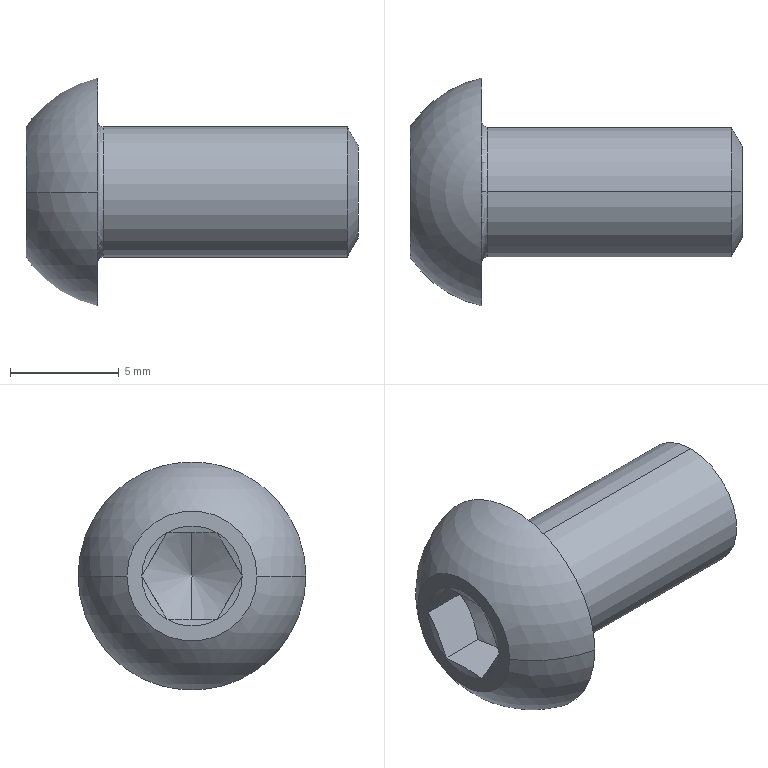Part | SolidWorks | features RevCut 2, Revolution 2, Cut 1, LPattern 1, RefAxis 1 | 1 solid | 25 faces | box 15.3 x 10.5 x 10.5 mm | volume 508.665 mm3 | cone 10 | plane 9 | torus 2 | sphere 2 | cylinder 2 | commonest cylinder face diameters 6 x2
STEP:
#1=CARTESIAN_POINT('',(0.,0.,2.134));
#2=VERTEX_POINT('',#1);
#3=CARTESIAN_POINT('',(0.,0.,-2.134));
#4=VERTEX_POINT('',#3);
#5=CARTESIAN_POINT('',(0.,0.,0.));
#6=DIRECTION('',(-1.,0.,0.));
#7=DIRECTION('',(0.,0.,1.));
#8=AXIS2_PLACEMENT_3D('',#5,#6,#7);
#9=CIRCLE('',#8,2.134);
#10=EDGE_CURVE('',#2,#4,#9,.T.);
#11=ORIENTED_EDGE('',*,*,#10,.T.);
#12=CARTESIAN_POINT('',(-0.5,0.,-3.));
#13=VERTEX_POINT('',#12);
#14=CARTESIAN_POINT('',(-0.5,0.,-3.));
#15=DIRECTION('',(-0.5,0.,-0.866));
#16=VECTOR('',#15,1000.);
#17=LINE('',#14,#16);
#18=EDGE_CURVE('',#4,#13,#17,.T.);
#19=ORIENTED_EDGE('',*,*,#18,.T.);
#20=CARTESIAN_POINT('',(-0.5,0.,3.));
#21=VERTEX_POINT('',#20);
#22=CARTESIAN_POINT('',(-0.5,0.,0.));
#23=DIRECTION('',(-1.,0.,0.));
#24=DIRECTION('',(0.,0.,1.));
#25=AXIS2_PLACEMENT_3D('',#22,#23,#24);
#26=CIRCLE('',#25,3.);
#27=EDGE_CURVE('',#21,#13,#26,.T.);
#28=ORIENTED_EDGE('',*,*,#27,.F.);
#29=CARTESIAN_POINT('',(-0.5,0.,3.));
#30=DIRECTION('',(-0.5,0.,0.866));
#31=VECTOR('',#30,1000.);
#32=LINE('',#29,#31);
#33=EDGE_CURVE('',#2,#21,#32,.T.);
#34=ORIENTED_EDGE('',*,*,#33,.F.);
#35=EDGE_LOOP('',(#11,#19,#28,#34));
#36=FACE_OUTER_BOUND('',#35,.T.);
#37=CARTESIAN_POINT('',(-0.5,0.,0.));
#38=DIRECTION('',(-1.,0.,0.));
#39=DIRECTION('',(0.,0.,1.));
#40=AXIS2_PLACEMENT_3D('',#37,#38,#39);
#41=CONICAL_SURFACE('',#40,3.,1.047);
#42=ADVANCED_FACE('',(#36),#41,.T.);
#43=CARTESIAN_POINT('',(-12.,0.,0.));
#44=VERTEX_POINT('',#43);
#45=CARTESIAN_POINT('',(-13.057,0.,2.));
#46=VERTEX_POINT('',#45);
#47=CARTESIAN_POINT('',(-13.22,0.,2.309));
#48=DIRECTION('',(-0.4671,0.,0.8842));
#49=VECTOR('',#48,1000.);
#50=LINE('',#47,#49);
#51=EDGE_CURVE('',#44,#46,#50,.T.);
#52=ORIENTED_EDGE('',*,*,#51,.F.);
#53=CARTESIAN_POINT('',(-13.057,0.,-2.));
#54=VERTEX_POINT('',#53);
#55=CARTESIAN_POINT('',(-13.22,0.,-2.309));
#56=DIRECTION('',(-0.4671,0.,-0.8842));
#57=VECTOR('',#56,1000.);
#58=LINE('',#55,#57);
#59=EDGE_CURVE('',#44,#54,#58,.T.);
#60=ORIENTED_EDGE('',*,*,#59,.T.);
#61=CARTESIAN_POINT('',(-13.22,-1.155,-2.));
#62=VERTEX_POINT('',#61);
#63=CARTESIAN_POINT('',(-13.057,0.,-2.));
#64=CARTESIAN_POINT('',(-13.057,-0.1946,-2.));
#65=CARTESIAN_POINT('',(-13.072,-0.3883,-2.));
#66=CARTESIAN_POINT('',(-13.129,-0.774,-2.));
#67=CARTESIAN_POINT('',(-13.17,-0.9664,-2.));
#68=CARTESIAN_POINT('',(-13.22,-1.155,-2.));
#69=B_SPLINE_CURVE_WITH_KNOTS('',3,(#63,#64,#65,#66,#67,#68),.UNSPECIFIED.,.F.,.F.,(4,2,4),(0.002255,0.002836,0.003416),.UNSPECIFIED.);
#70=EDGE_CURVE('',#54,#62,#69,.T.);
#71=ORIENTED_EDGE('',*,*,#70,.T.);
#72=CARTESIAN_POINT('',(-13.22,-2.309,0.));
#73=VERTEX_POINT('',#72);
#74=CARTESIAN_POINT('',(-13.22,-1.155,-2.));
#75=CARTESIAN_POINT('',(-13.12,-1.344,-1.672));
#76=CARTESIAN_POINT('',(-13.057,-1.535,-1.341));
#77=CARTESIAN_POINT('',(-13.056,-1.927,-0.6622));
#78=CARTESIAN_POINT('',(-13.12,-2.12,-0.3279));
#79=CARTESIAN_POINT('',(-13.22,-2.309,0.));
#80=B_SPLINE_CURVE_WITH_KNOTS('',3,(#74,#75,#76,#77,#78,#79),.UNSPECIFIED.,.F.,.F.,(4,2,4),(0.000000237,0.001165,0.002329),.UNSPECIFIED.);
#81=EDGE_CURVE('',#62,#73,#80,.T.);
#82=ORIENTED_EDGE('',*,*,#81,.T.);
#83=CARTESIAN_POINT('',(-13.22,-1.155,2.));
#84=VERTEX_POINT('',#83);
#85=CARTESIAN_POINT('',(-13.22,-2.309,0.));
#86=CARTESIAN_POINT('',(-13.12,-2.12,0.3276));
#87=CARTESIAN_POINT('',(-13.057,-1.929,0.6595));
#88=CARTESIAN_POINT('',(-13.056,-1.537,1.338));
#89=CARTESIAN_POINT('',(-13.12,-1.344,1.672));
#90=CARTESIAN_POINT('',(-13.22,-1.155,2.));
#91=B_SPLINE_CURVE_WITH_KNOTS('',3,(#85,#86,#87,#88,#89,#90),.UNSPECIFIED.,.F.,.F.,(4,2,4),(0.000000237,0.001165,0.002329),.UNSPECIFIED.);
#92=EDGE_CURVE('',#73,#84,#91,.T.);
#93=ORIENTED_EDGE('',*,*,#92,.T.);
#94=CARTESIAN_POINT('',(-13.22,-1.155,2.));
#95=CARTESIAN_POINT('',(-13.17,-0.9664,2.));
#96=CARTESIAN_POINT('',(-13.129,-0.774,2.));
#97=CARTESIAN_POINT('',(-13.072,-0.3883,2.));
#98=CARTESIAN_POINT('',(-13.057,-0.1946,2.));
#99=CARTESIAN_POINT('',(-13.057,0.,2.));
#100=B_SPLINE_CURVE_WITH_KNOTS('',3,(#94,#95,#96,#97,#98,#99),.UNSPECIFIED.,.F.,.F.,(4,2,4),(0.001973,0.002555,0.003138),.UNSPECIFIED.);
#101=EDGE_CURVE('',#84,#46,#100,.T.);
#102=ORIENTED_EDGE('',*,*,#101,.T.);
#103=EDGE_LOOP('',(#52,#60,#71,#82,#93,#102));
#104=FACE_OUTER_BOUND('',#103,.T.);
#105=CARTESIAN_POINT('',(-13.22,0.,0.));
#106=DIRECTION('',(-1.,0.,0.));
#107=DIRECTION('',(0.,0.,1.));
#108=AXIS2_PLACEMENT_3D('',#105,#106,#107);
#109=CONICAL_SURFACE('',#108,2.309,1.085);
#110=ADVANCED_FACE('',(#104),#109,.F.);
#111=CARTESIAN_POINT('',(-12.,0.,-3.25));
#112=VERTEX_POINT('',#111);
#113=CARTESIAN_POINT('',(-12.,0.,3.25));
#114=VERTEX_POINT('',#113);
#115=CARTESIAN_POINT('',(-12.,0.,0.));
#116=DIRECTION('',(-1.,0.,0.));
#117=DIRECTION('',(0.,0.,1.));
#118=AXIS2_PLACEMENT_3D('',#115,#116,#117);
#119=CIRCLE('',#118,3.25);
#120=EDGE_CURVE('',#112,#114,#119,.T.);
#121=ORIENTED_EDGE('',*,*,#120,.F.);
#122=CARTESIAN_POINT('',(-11.75,0.,-3.));
#123=VERTEX_POINT('',#122);
#124=CARTESIAN_POINT('',(-11.75,0.,-3.25));
#125=DIRECTION('',(0.,1.,0.));
#126=DIRECTION('',(0.,0.,1.));
#127=AXIS2_PLACEMENT_3D('',#124,#125,#126);
#128=CIRCLE('',#127,0.25);
#129=EDGE_CURVE('',#112,#123,#128,.T.);
#130=ORIENTED_EDGE('',*,*,#129,.T.);
#131=CARTESIAN_POINT('',(-11.75,0.,3.));
#132=VERTEX_POINT('',#131);
#133=CARTESIAN_POINT('',(-11.75,0.,0.));
#134=DIRECTION('',(-1.,0.,0.));
#135=DIRECTION('',(0.,0.,1.));
#136=AXIS2_PLACEMENT_3D('',#133,#134,#135);
#137=CIRCLE('',#136,3.);
#138=EDGE_CURVE('',#123,#132,#137,.T.);
#139=ORIENTED_EDGE('',*,*,#138,.T.);
#140=CARTESIAN_POINT('',(-11.75,0.,3.25));
#141=DIRECTION('',(0.,-1.,0.));
#142=DIRECTION('',(0.,0.,-1.));
#143=AXIS2_PLACEMENT_3D('',#140,#141,#142);
#144=CIRCLE('',#143,0.25);
#145=EDGE_CURVE('',#114,#132,#144,.T.);
#146=ORIENTED_EDGE('',*,*,#145,.F.);
#147=EDGE_LOOP('',(#121,#130,#139,#146));
#148=FACE_OUTER_BOUND('',#147,.T.);
#149=CARTESIAN_POINT('',(-11.75,0.,0.));
#150=DIRECTION('',(-1.,0.,0.));
#151=DIRECTION('',(0.,0.,1.));
#152=AXIS2_PLACEMENT_3D('',#149,#150,#151);
#153=TOROIDAL_SURFACE('',#152,3.25,0.25);
#154=ADVANCED_FACE('',(#148),#153,.F.);
#155=CARTESIAN_POINT('',(-12.,5.25,0.));
#156=VERTEX_POINT('',#155);
#157=CARTESIAN_POINT('',(-12.,-5.25,0.));
#158=VERTEX_POINT('',#157);
#159=CARTESIAN_POINT('',(-12.,0.,0.));
#160=DIRECTION('',(-1.,0.,0.));
#161=DIRECTION('',(0.,0.,1.));
#162=AXIS2_PLACEMENT_3D('',#159,#160,#161);
#163=CIRCLE('',#162,5.25);
#164=EDGE_CURVE('',#156,#158,#163,.T.);
#165=ORIENTED_EDGE('',*,*,#164,.T.);
#166=CARTESIAN_POINT('',(-15.3,-3.,0.));
#167=VERTEX_POINT('',#166);
#168=CARTESIAN_POINT('',(-10.838,0.,0.));
#169=DIRECTION('',(0.,0.,-1.));
#170=DIRECTION('',(0.,1.,0.));
#171=AXIS2_PLACEMENT_3D('',#168,#169,#170);
#172=CIRCLE('',#171,5.377);
#173=EDGE_CURVE('',#158,#167,#172,.T.);
#174=ORIENTED_EDGE('',*,*,#173,.T.);
#175=CARTESIAN_POINT('',(-15.3,3.,0.));
#176=VERTEX_POINT('',#175);
#177=CARTESIAN_POINT('',(-15.3,0.,0.));
#178=DIRECTION('',(-1.,0.,0.));
#179=DIRECTION('',(0.,0.,1.));
#180=AXIS2_PLACEMENT_3D('',#177,#178,#179);
#181=CIRCLE('',#180,3.);
#182=EDGE_CURVE('',#176,#167,#181,.T.);
#183=ORIENTED_EDGE('',*,*,#182,.F.);
#184=CARTESIAN_POINT('',(-10.838,0.,0.));
#185=DIRECTION('',(0.,0.,1.));
#186=DIRECTION('',(1.,0.,0.));
#187=AXIS2_PLACEMENT_3D('',#184,#185,#186);
#188=CIRCLE('',#187,5.377);
#189=EDGE_CURVE('',#156,#176,#188,.T.);
#190=ORIENTED_EDGE('',*,*,#189,.F.);
#191=EDGE_LOOP('',(#165,#174,#183,#190));
#192=FACE_OUTER_BOUND('',#191,.T.);
#193=CARTESIAN_POINT('',(-10.838,0.,0.));
#194=DIRECTION('',(0.,0.,-1.));
#195=DIRECTION('',(0.,1.,0.));
#196=AXIS2_PLACEMENT_3D('',#193,#194,#195);
#197=SPHERICAL_SURFACE('',#196,5.377);
#198=ADVANCED_FACE('',(#192),#197,.T.);
#199=ORIENTED_EDGE('',*,*,#27,.T.);
#200=CARTESIAN_POINT('',(-15.3,0.,-3.));
#201=DIRECTION('',(-1.,0.,0.));
#202=VECTOR('',#201,1000.);
#203=LINE('',#200,#202);
#204=EDGE_CURVE('',#13,#123,#203,.T.);
#205=ORIENTED_EDGE('',*,*,#204,.T.);
#206=CARTESIAN_POINT('',(-11.75,0.,0.));
#207=DIRECTION('',(-1.,0.,0.));
#208=DIRECTION('',(0.,0.,1.));
#209=AXIS2_PLACEMENT_3D('',#206,#207,#208);
#210=CIRCLE('',#209,3.);
#211=EDGE_CURVE('',#132,#123,#210,.T.);
#212=ORIENTED_EDGE('',*,*,#211,.F.);
#213=CARTESIAN_POINT('',(-15.3,0.,3.));
#214=DIRECTION('',(-1.,0.,0.));
#215=VECTOR('',#214,1000.);
#216=LINE('',#213,#215);
#217=EDGE_CURVE('',#21,#132,#216,.T.);
#218=ORIENTED_EDGE('',*,*,#217,.F.);
#219=EDGE_LOOP('',(#199,#205,#212,#218));
#220=FACE_OUTER_BOUND('',#219,.T.);
#221=CARTESIAN_POINT('',(-15.3,0.,0.));
#222=DIRECTION('',(-1.,0.,0.));
#223=DIRECTION('',(0.,0.,1.));
#224=AXIS2_PLACEMENT_3D('',#221,#222,#223);
#225=CYLINDRICAL_SURFACE('',#224,3.);
#226=ADVANCED_FACE('',(#220),#225,.T.);
#227=ORIENTED_EDGE('',*,*,#204,.F.);
#228=CARTESIAN_POINT('',(-0.5,0.,0.));
#229=DIRECTION('',(-1.,0.,0.));
#230=DIRECTION('',(0.,0.,1.));
#231=AXIS2_PLACEMENT_3D('',#228,#229,#230);
#232=CIRCLE('',#231,3.);
#233=EDGE_CURVE('',#13,#21,#232,.T.);
#234=ORIENTED_EDGE('',*,*,#233,.T.);
#235=ORIENTED_EDGE('',*,*,#217,.T.);
#236=ORIENTED_EDGE('',*,*,#138,.F.);
#237=EDGE_LOOP('',(#227,#234,#235,#236));
#238=FACE_OUTER_BOUND('',#237,.T.);
#239=CARTESIAN_POINT('',(-15.3,0.,0.));
#240=DIRECTION('',(-1.,0.,0.));
#241=DIRECTION('',(0.,0.,1.));
#242=AXIS2_PLACEMENT_3D('',#239,#240,#241);
#243=CYLINDRICAL_SURFACE('',#242,3.);
#244=ADVANCED_FACE('',(#238),#243,.T.);
#245=ORIENTED_EDGE('',*,*,#182,.T.);
#246=CARTESIAN_POINT('',(-15.3,0.,0.));
#247=DIRECTION('',(-1.,0.,0.));
#248=DIRECTION('',(0.,0.,1.));
#249=AXIS2_PLACEMENT_3D('',#246,#247,#248);
#250=CIRCLE('',#249,3.);
#251=EDGE_CURVE('',#167,#176,#250,.T.);
#252=ORIENTED_EDGE('',*,*,#251,.T.);
#253=EDGE_LOOP('',(#245,#252));
#254=FACE_OUTER_BOUND('',#253,.T.);
#255=CARTESIAN_POINT('',(-15.3,-1.155,-2.));
#256=VERTEX_POINT('',#255);
#257=CARTESIAN_POINT('',(-15.3,-2.309,0.));
#258=VERTEX_POINT('',#257);
#259=CARTESIAN_POINT('',(-15.3,0.,0.));
#260=DIRECTION('',(-1.,0.,0.));
#261=DIRECTION('',(0.,0.,-1.));
#262=AXIS2_PLACEMENT_3D('',#259,#260,#261);
#263=CIRCLE('',#262,2.309);
#264=EDGE_CURVE('',#256,#258,#263,.T.);
#265=ORIENTED_EDGE('',*,*,#264,.F.);
#266=CARTESIAN_POINT('',(-15.3,1.155,-2.));
#267=VERTEX_POINT('',#266);
#268=CARTESIAN_POINT('',(-15.3,0.,0.));
#269=DIRECTION('',(-1.,0.,0.));
#270=DIRECTION('',(0.,0.,-1.));
#271=AXIS2_PLACEMENT_3D('',#268,#269,#270);
#272=CIRCLE('',#271,2.309);
#273=EDGE_CURVE('',#267,#256,#272,.T.);
#274=ORIENTED_EDGE('',*,*,#273,.F.);
#275=CARTESIAN_POINT('',(-15.3,2.309,0.));
#276=VERTEX_POINT('',#275);
#277=CARTESIAN_POINT('',(-15.3,0.,0.));
#278=DIRECTION('',(-1.,0.,0.));
#279=DIRECTION('',(0.,0.,-1.));
#280=AXIS2_PLACEMENT_3D('',#277,#278,#279);
#281=CIRCLE('',#280,2.309);
#282=EDGE_CURVE('',#276,#267,#281,.T.);
#283=ORIENTED_EDGE('',*,*,#282,.F.);
#284=CARTESIAN_POINT('',(-15.3,1.155,2.));
#285=VERTEX_POINT('',#284);
#286=CARTESIAN_POINT('',(-15.3,0.,0.));
#287=DIRECTION('',(-1.,0.,0.));
#288=DIRECTION('',(0.,0.,-1.));
#289=AXIS2_PLACEMENT_3D('',#286,#287,#288);
#290=CIRCLE('',#289,2.309);
#291=EDGE_CURVE('',#285,#276,#290,.T.);
#292=ORIENTED_EDGE('',*,*,#291,.F.);
#293=CARTESIAN_POINT('',(-15.3,-1.155,2.));
#294=VERTEX_POINT('',#293);
#295=CARTESIAN_POINT('',(-15.3,0.,0.));
#296=DIRECTION('',(-1.,0.,0.));
#297=DIRECTION('',(0.,0.,-1.));
#298=AXIS2_PLACEMENT_3D('',#295,#296,#297);
#299=CIRCLE('',#298,2.309);
#300=EDGE_CURVE('',#294,#285,#299,.T.);
#301=ORIENTED_EDGE('',*,*,#300,.F.);
#302=CARTESIAN_POINT('',(-15.3,0.,0.));
#303=DIRECTION('',(-1.,0.,0.));
#304=DIRECTION('',(0.,-1.,0.));
#305=AXIS2_PLACEMENT_3D('',#302,#303,#304);
#306=CIRCLE('',#305,2.309);
#307=EDGE_CURVE('',#258,#294,#306,.T.);
#308=ORIENTED_EDGE('',*,*,#307,.F.);
#309=EDGE_LOOP('',(#265,#274,#283,#292,#301,#308));
#310=FACE_BOUND('',#309,.T.);
#311=CARTESIAN_POINT('',(-15.3,0.,0.));
#312=DIRECTION('',(1.,0.,0.));
#313=DIRECTION('',(0.,0.,-1.));
#314=AXIS2_PLACEMENT_3D('',#311,#312,#313);
#315=PLANE('',#314);
#316=ADVANCED_FACE('',(#254,#310),#315,.F.);
#317=ORIENTED_EDGE('',*,*,#173,.F.);
#318=CARTESIAN_POINT('',(-12.,0.,0.));
#319=DIRECTION('',(-1.,0.,0.));
#320=DIRECTION('',(0.,0.,1.));
#321=AXIS2_PLACEMENT_3D('',#318,#319,#320);
#322=CIRCLE('',#321,5.25);
#323=EDGE_CURVE('',#158,#156,#322,.T.);
#324=ORIENTED_EDGE('',*,*,#323,.T.);
#325=ORIENTED_EDGE('',*,*,#189,.T.);
#326=ORIENTED_EDGE('',*,*,#251,.F.);
#327=EDGE_LOOP('',(#317,#324,#325,#326));
#328=FACE_OUTER_BOUND('',#327,.T.);
#329=CARTESIAN_POINT('',(-10.838,0.,0.));
#330=DIRECTION('',(0.,0.,-1.));
#331=DIRECTION('',(0.,1.,0.));
#332=AXIS2_PLACEMENT_3D('',#329,#330,#331);
#333=SPHERICAL_SURFACE('',#332,5.377);
#334=ADVANCED_FACE('',(#328),#333,.T.);
#335=ORIENTED_EDGE('',*,*,#164,.F.);
#336=ORIENTED_EDGE('',*,*,#323,.F.);
#337=EDGE_LOOP('',(#335,#336));
#338=FACE_OUTER_BOUND('',#337,.T.);
#339=CARTESIAN_POINT('',(-12.,0.,0.));
#340=DIRECTION('',(-1.,0.,0.));
#341=DIRECTION('',(0.,0.,1.));
#342=AXIS2_PLACEMENT_3D('',#339,#340,#341);
#343=CIRCLE('',#342,3.25);
#344=EDGE_CURVE('',#114,#112,#343,.T.);
#345=ORIENTED_EDGE('',*,*,#344,.T.);
#346=ORIENTED_EDGE('',*,*,#120,.T.);
#347=EDGE_LOOP('',(#345,#346));
#348=FACE_BOUND('',#347,.T.);
#349=CARTESIAN_POINT('',(-12.,3.25,0.));
#350=DIRECTION('',(-1.,0.,0.));
#351=DIRECTION('',(0.,0.,1.));
#352=AXIS2_PLACEMENT_3D('',#349,#350,#351);
#353=PLANE('',#352);
#354=ADVANCED_FACE('',(#338,#348),#353,.F.);
#355=ORIENTED_EDGE('',*,*,#129,.F.);
#356=ORIENTED_EDGE('',*,*,#344,.F.);
#357=ORIENTED_EDGE('',*,*,#145,.T.);
#358=ORIENTED_EDGE('',*,*,#211,.T.);
#359=EDGE_LOOP('',(#355,#356,#357,#358));
#360=FACE_OUTER_BOUND('',#359,.T.);
#361=CARTESIAN_POINT('',(-11.75,0.,0.));
#362=DIRECTION('',(-1.,0.,0.));
#363=DIRECTION('',(0.,0.,1.));
#364=AXIS2_PLACEMENT_3D('',#361,#362,#363);
#365=TOROIDAL_SURFACE('',#364,3.25,0.25);
#366=ADVANCED_FACE('',(#360),#365,.F.);
#367=CARTESIAN_POINT('',(-15.3,-1.155,-2.));
#368=CARTESIAN_POINT('',(-15.252,-0.7703,-2.));
#369=CARTESIAN_POINT('',(-15.222,-0.3832,-2.));
#370=CARTESIAN_POINT('',(-15.222,0.3869,-2.));
#371=CARTESIAN_POINT('',(-15.252,0.7711,-2.));
#372=CARTESIAN_POINT('',(-15.3,1.155,-2.));
#373=B_SPLINE_CURVE_WITH_KNOTS('',3,(#367,#368,#369,#370,#371,#372),.UNSPECIFIED.,.F.,.F.,(4,2,4),(0.001892,0.003053,0.004215),.UNSPECIFIED.);
#374=EDGE_CURVE('',#256,#267,#373,.T.);
#375=ORIENTED_EDGE('',*,*,#374,.T.);
#376=ORIENTED_EDGE('',*,*,#273,.T.);
#377=EDGE_LOOP('',(#375,#376));
#378=FACE_OUTER_BOUND('',#377,.T.);
#379=CARTESIAN_POINT('',(-1014.72,0.,0.));
#380=DIRECTION('',(-1.,0.,0.));
#381=DIRECTION('',(0.,-1.,0.));
#382=AXIS2_PLACEMENT_3D('',#379,#380,#381);
#383=CONICAL_SURFACE('',#382,3981.726,1.325);
#384=ADVANCED_FACE('',(#378),#383,.F.);
#385=CARTESIAN_POINT('',(-15.3,1.155,-2.));
#386=CARTESIAN_POINT('',(-15.252,1.347,-1.667));
#387=CARTESIAN_POINT('',(-15.193,1.732,-1.));
#388=CARTESIAN_POINT('',(-15.252,2.117,-0.3333));
#389=CARTESIAN_POINT('',(-15.3,2.309,0.));
#390=B_SPLINE_CURVE_WITH_KNOTS('',3,(#385,#386,#387,#388,#389),.UNSPECIFIED.,.F.,.F.,(4,1,4),(0.000000231,0.001155,0.00231),.UNSPECIFIED.);
#391=EDGE_CURVE('',#267,#276,#390,.T.);
#392=ORIENTED_EDGE('',*,*,#391,.T.);
#393=ORIENTED_EDGE('',*,*,#282,.T.);
#394=EDGE_LOOP('',(#392,#393));
#395=FACE_OUTER_BOUND('',#394,.T.);
#396=CARTESIAN_POINT('',(-1014.72,0.,0.));
#397=DIRECTION('',(-1.,0.,0.));
#398=DIRECTION('',(0.,-1.,0.));
#399=AXIS2_PLACEMENT_3D('',#396,#397,#398);
#400=CONICAL_SURFACE('',#399,3981.726,1.325);
#401=ADVANCED_FACE('',(#395),#400,.F.);
#402=CARTESIAN_POINT('',(-15.3,2.309,0.));
#403=CARTESIAN_POINT('',(-15.252,2.117,0.3333));
#404=CARTESIAN_POINT('',(-15.193,1.732,1.));
#405=CARTESIAN_POINT('',(-15.252,1.347,1.667));
#406=CARTESIAN_POINT('',(-15.3,1.155,2.));
#407=B_SPLINE_CURVE_WITH_KNOTS('',3,(#402,#403,#404,#405,#406),.UNSPECIFIED.,.F.,.F.,(4,1,4),(0.000000231,0.001155,0.00231),.UNSPECIFIED.);
#408=EDGE_CURVE('',#276,#285,#407,.T.);
#409=ORIENTED_EDGE('',*,*,#408,.T.);
#410=ORIENTED_EDGE('',*,*,#291,.T.);
#411=EDGE_LOOP('',(#409,#410));
#412=FACE_OUTER_BOUND('',#411,.T.);
#413=CARTESIAN_POINT('',(-1014.72,0.,0.));
#414=DIRECTION('',(-1.,0.,0.));
#415=DIRECTION('',(0.,-1.,0.));
#416=AXIS2_PLACEMENT_3D('',#413,#414,#415);
#417=CONICAL_SURFACE('',#416,3981.726,1.325);
#418=ADVANCED_FACE('',(#412),#417,.F.);
#419=CARTESIAN_POINT('',(-15.3,1.155,2.));
#420=CARTESIAN_POINT('',(-15.252,0.7711,2.));
#421=CARTESIAN_POINT('',(-15.222,0.3869,2.));
#422=CARTESIAN_POINT('',(-15.222,-0.3832,2.));
#423=CARTESIAN_POINT('',(-15.252,-0.7703,2.));
#424=CARTESIAN_POINT('',(-15.3,-1.155,2.));
#425=B_SPLINE_CURVE_WITH_KNOTS('',3,(#419,#420,#421,#422,#423,#424),.UNSPECIFIED.,.F.,.F.,(4,2,4),(0.004742,0.005901,0.007061),.UNSPECIFIED.);
#426=EDGE_CURVE('',#285,#294,#425,.T.);
#427=ORIENTED_EDGE('',*,*,#426,.T.);
#428=ORIENTED_EDGE('',*,*,#300,.T.);
#429=EDGE_LOOP('',(#427,#428));
#430=FACE_OUTER_BOUND('',#429,.T.);
#431=CARTESIAN_POINT('',(-1014.72,0.,0.));
#432=DIRECTION('',(-1.,0.,0.));
#433=DIRECTION('',(0.,-1.,0.));
#434=AXIS2_PLACEMENT_3D('',#431,#432,#433);
#435=CONICAL_SURFACE('',#434,3981.726,1.325);
#436=ADVANCED_FACE('',(#430),#435,.F.);
#437=CARTESIAN_POINT('',(-15.3,-1.155,2.));
#438=CARTESIAN_POINT('',(-15.252,-1.347,1.667));
#439=CARTESIAN_POINT('',(-15.193,-1.732,1.));
#440=CARTESIAN_POINT('',(-15.252,-2.117,0.3333));
#441=CARTESIAN_POINT('',(-15.3,-2.309,0.));
#442=B_SPLINE_CURVE_WITH_KNOTS('',3,(#437,#438,#439,#440,#441),.UNSPECIFIED.,.F.,.F.,(4,1,4),(0.000000231,0.001155,0.00231),.UNSPECIFIED.);
#443=EDGE_CURVE('',#294,#258,#442,.T.);
#444=ORIENTED_EDGE('',*,*,#443,.T.);
#445=ORIENTED_EDGE('',*,*,#307,.T.);
#446=EDGE_LOOP('',(#444,#445));
#447=FACE_OUTER_BOUND('',#446,.T.);
#448=CARTESIAN_POINT('',(-1014.72,0.,0.));
#449=DIRECTION('',(-1.,0.,0.));
#450=DIRECTION('',(0.,-1.,0.));
#451=AXIS2_PLACEMENT_3D('',#448,#449,#450);
#452=CONICAL_SURFACE('',#451,3981.726,1.325);
#453=ADVANCED_FACE('',(#447),#452,.F.);
#454=CARTESIAN_POINT('',(-15.3,-2.309,0.));
#455=CARTESIAN_POINT('',(-15.252,-2.117,-0.3333));
#456=CARTESIAN_POINT('',(-15.193,-1.732,-1.));
#457=CARTESIAN_POINT('',(-15.252,-1.347,-1.667));
#458=CARTESIAN_POINT('',(-15.3,-1.155,-2.));
#459=B_SPLINE_CURVE_WITH_KNOTS('',3,(#454,#455,#456,#457,#458),.UNSPECIFIED.,.F.,.F.,(4,1,4),(0.000000231,0.001155,0.00231),.UNSPECIFIED.);
#460=EDGE_CURVE('',#258,#256,#459,.T.);
#461=ORIENTED_EDGE('',*,*,#460,.T.);
#462=ORIENTED_EDGE('',*,*,#264,.T.);
#463=EDGE_LOOP('',(#461,#462));
#464=FACE_OUTER_BOUND('',#463,.T.);
#465=CARTESIAN_POINT('',(-1014.72,0.,0.));
#466=DIRECTION('',(-1.,0.,0.));
#467=DIRECTION('',(0.,-1.,0.));
#468=AXIS2_PLACEMENT_3D('',#465,#466,#467);
#469=CONICAL_SURFACE('',#468,3981.726,1.325);
#470=ADVANCED_FACE('',(#464),#469,.F.);
#471=ORIENTED_EDGE('',*,*,#59,.F.);
#472=ORIENTED_EDGE('',*,*,#51,.T.);
#473=CARTESIAN_POINT('',(-13.22,1.155,2.));
#474=VERTEX_POINT('',#473);
#475=CARTESIAN_POINT('',(-13.057,0.,2.));
#476=CARTESIAN_POINT('',(-13.057,0.1949,2.));
#477=CARTESIAN_POINT('',(-13.072,0.3921,2.));
#478=CARTESIAN_POINT('',(-13.129,0.7778,2.));
#479=CARTESIAN_POINT('',(-13.171,0.9674,2.));
#480=CARTESIAN_POINT('',(-13.22,1.155,2.));
#481=B_SPLINE_CURVE_WITH_KNOTS('',3,(#475,#476,#477,#478,#479,#480),.UNSPECIFIED.,.F.,.F.,(4,2,4),(0.003138,0.003721,0.004305),.UNSPECIFIED.);
#482=EDGE_CURVE('',#46,#474,#481,.T.);
#483=ORIENTED_EDGE('',*,*,#482,.T.);
#484=CARTESIAN_POINT('',(-13.22,2.309,0.));
#485=VERTEX_POINT('',#484);
#486=CARTESIAN_POINT('',(-13.22,1.155,2.));
#487=CARTESIAN_POINT('',(-13.12,1.344,1.672));
#488=CARTESIAN_POINT('',(-13.057,1.535,1.341));
#489=CARTESIAN_POINT('',(-13.056,1.927,0.6622));
#490=CARTESIAN_POINT('',(-13.12,2.12,0.3279));
#491=CARTESIAN_POINT('',(-13.22,2.309,0.));
#492=B_SPLINE_CURVE_WITH_KNOTS('',3,(#486,#487,#488,#489,#490,#491),.UNSPECIFIED.,.F.,.F.,(4,2,4),(0.000000237,0.001165,0.002329),.UNSPECIFIED.);
#493=EDGE_CURVE('',#474,#485,#492,.T.);
#494=ORIENTED_EDGE('',*,*,#493,.T.);
#495=CARTESIAN_POINT('',(-13.22,1.155,-2.));
#496=VERTEX_POINT('',#495);
#497=CARTESIAN_POINT('',(-13.22,2.309,0.));
#498=CARTESIAN_POINT('',(-13.12,2.12,-0.3276));
#499=CARTESIAN_POINT('',(-13.057,1.929,-0.6595));
#500=CARTESIAN_POINT('',(-13.056,1.537,-1.338));
#501=CARTESIAN_POINT('',(-13.12,1.344,-1.672));
#502=CARTESIAN_POINT('',(-13.22,1.155,-2.));
#503=B_SPLINE_CURVE_WITH_KNOTS('',3,(#497,#498,#499,#500,#501,#502),.UNSPECIFIED.,.F.,.F.,(4,2,4),(0.000000237,0.001165,0.002329),.UNSPECIFIED.);
#504=EDGE_CURVE('',#485,#496,#503,.T.);
#505=ORIENTED_EDGE('',*,*,#504,.T.);
#506=CARTESIAN_POINT('',(-13.22,1.155,-2.));
#507=CARTESIAN_POINT('',(-13.171,0.9674,-2.));
#508=CARTESIAN_POINT('',(-13.129,0.7778,-2.));
#509=CARTESIAN_POINT('',(-13.072,0.3921,-2.));
#510=CARTESIAN_POINT('',(-13.057,0.1949,-2.));
#511=CARTESIAN_POINT('',(-13.057,0.,-2.));
#512=B_SPLINE_CURVE_WITH_KNOTS('',3,(#506,#507,#508,#509,#510,#511),.UNSPECIFIED.,.F.,.F.,(4,2,4),(0.001093,0.001674,0.002255),.UNSPECIFIED.);
#513=EDGE_CURVE('',#496,#54,#512,.T.);
#514=ORIENTED_EDGE('',*,*,#513,.T.);
#515=EDGE_LOOP('',(#471,#472,#483,#494,#505,#514));
#516=FACE_OUTER_BOUND('',#515,.T.);
#517=CARTESIAN_POINT('',(-13.22,0.,0.));
#518=DIRECTION('',(-1.,0.,0.));
#519=DIRECTION('',(0.,0.,1.));
#520=AXIS2_PLACEMENT_3D('',#517,#518,#519);
#521=CONICAL_SURFACE('',#520,2.309,1.085);
#522=ADVANCED_FACE('',(#516),#521,.F.);
#523=ORIENTED_EDGE('',*,*,#391,.F.);
#524=CARTESIAN_POINT('',(-12.,1.155,-2.));
#525=DIRECTION('',(-1.,0.,0.));
#526=VECTOR('',#525,1000.);
#527=LINE('',#524,#526);
#528=EDGE_CURVE('',#496,#267,#527,.T.);
#529=ORIENTED_EDGE('',*,*,#528,.F.);
#530=ORIENTED_EDGE('',*,*,#504,.F.);
#531=CARTESIAN_POINT('',(-12.,2.309,0.));
#532=DIRECTION('',(-1.,0.,0.));
#533=VECTOR('',#532,1000.);
#534=LINE('',#531,#533);
#535=EDGE_CURVE('',#485,#276,#534,.T.);
#536=ORIENTED_EDGE('',*,*,#535,.T.);
#537=EDGE_LOOP('',(#523,#529,#530,#536));
#538=FACE_OUTER_BOUND('',#537,.T.);
#539=CARTESIAN_POINT('',(-12.,2.309,0.));
#540=DIRECTION('',(0.,0.866,-0.5));
#541=DIRECTION('',(0.,0.5,0.866));
#542=AXIS2_PLACEMENT_3D('',#539,#540,#541);
#543=PLANE('',#542);
#544=ADVANCED_FACE('',(#538),#543,.F.);
#545=ORIENTED_EDGE('',*,*,#374,.F.);
#546=CARTESIAN_POINT('',(-12.,-1.155,-2.));
#547=DIRECTION('',(-1.,0.,0.));
#548=VECTOR('',#547,1000.);
#549=LINE('',#546,#548);
#550=EDGE_CURVE('',#62,#256,#549,.T.);
#551=ORIENTED_EDGE('',*,*,#550,.F.);
#552=ORIENTED_EDGE('',*,*,#70,.F.);
#553=ORIENTED_EDGE('',*,*,#513,.F.);
#554=ORIENTED_EDGE('',*,*,#528,.T.);
#555=EDGE_LOOP('',(#545,#551,#552,#553,#554));
#556=FACE_OUTER_BOUND('',#555,.T.);
#557=CARTESIAN_POINT('',(-12.,1.155,-2.));
#558=DIRECTION('',(0.,0.,-1.));
#559=DIRECTION('',(-1.,0.,0.));
#560=AXIS2_PLACEMENT_3D('',#557,#558,#559);
#561=PLANE('',#560);
#562=ADVANCED_FACE('',(#556),#561,.F.);
#563=ORIENTED_EDGE('',*,*,#460,.F.);
#564=CARTESIAN_POINT('',(-12.,-2.309,0.));
#565=DIRECTION('',(-1.,0.,0.));
#566=VECTOR('',#565,1000.);
#567=LINE('',#564,#566);
#568=EDGE_CURVE('',#73,#258,#567,.T.);
#569=ORIENTED_EDGE('',*,*,#568,.F.);
#570=ORIENTED_EDGE('',*,*,#81,.F.);
#571=ORIENTED_EDGE('',*,*,#550,.T.);
#572=EDGE_LOOP('',(#563,#569,#570,#571));
#573=FACE_OUTER_BOUND('',#572,.T.);
#574=CARTESIAN_POINT('',(-12.,-1.155,-2.));
#575=DIRECTION('',(0.,-0.866,-0.5));
#576=DIRECTION('',(0.,0.5,-0.866));
#577=AXIS2_PLACEMENT_3D('',#574,#575,#576);
#578=PLANE('',#577);
#579=ADVANCED_FACE('',(#573),#578,.F.);
#580=ORIENTED_EDGE('',*,*,#443,.F.);
#581=CARTESIAN_POINT('',(-12.,-1.155,2.));
#582=DIRECTION('',(-1.,0.,0.));
#583=VECTOR('',#582,1000.);
#584=LINE('',#581,#583);
#585=EDGE_CURVE('',#84,#294,#584,.T.);
#586=ORIENTED_EDGE('',*,*,#585,.F.);
#587=ORIENTED_EDGE('',*,*,#92,.F.);
#588=ORIENTED_EDGE('',*,*,#568,.T.);
#589=EDGE_LOOP('',(#580,#586,#587,#588));
#590=FACE_OUTER_BOUND('',#589,.T.);
#591=CARTESIAN_POINT('',(-12.,-2.309,0.));
#592=DIRECTION('',(0.,-0.866,0.5));
#593=DIRECTION('',(0.,-0.5,-0.866));
#594=AXIS2_PLACEMENT_3D('',#591,#592,#593);
#595=PLANE('',#594);
#596=ADVANCED_FACE('',(#590),#595,.F.);
#597=ORIENTED_EDGE('',*,*,#426,.F.);
#598=CARTESIAN_POINT('',(-12.,1.155,2.));
#599=DIRECTION('',(-1.,0.,0.));
#600=VECTOR('',#599,1000.);
#601=LINE('',#598,#600);
#602=EDGE_CURVE('',#474,#285,#601,.T.);
#603=ORIENTED_EDGE('',*,*,#602,.F.);
#604=ORIENTED_EDGE('',*,*,#482,.F.);
#605=ORIENTED_EDGE('',*,*,#101,.F.);
#606=ORIENTED_EDGE('',*,*,#585,.T.);
#607=EDGE_LOOP('',(#597,#603,#604,#605,#606));
#608=FACE_OUTER_BOUND('',#607,.T.);
#609=CARTESIAN_POINT('',(-12.,-1.155,2.));
#610=DIRECTION('',(0.,0.,1.));
#611=DIRECTION('',(0.,-1.,0.));
#612=AXIS2_PLACEMENT_3D('',#609,#610,#611);
#613=PLANE('',#612);
#614=ADVANCED_FACE('',(#608),#613,.F.);
#615=ORIENTED_EDGE('',*,*,#408,.F.);
#616=ORIENTED_EDGE('',*,*,#535,.F.);
#617=ORIENTED_EDGE('',*,*,#493,.F.);
#618=ORIENTED_EDGE('',*,*,#602,.T.);
#619=EDGE_LOOP('',(#615,#616,#617,#618));
#620=FACE_OUTER_BOUND('',#619,.T.);
#621=CARTESIAN_POINT('',(-12.,1.155,2.));
#622=DIRECTION('',(0.,0.866,0.5));
#623=DIRECTION('',(0.,-0.5,0.866));
#624=AXIS2_PLACEMENT_3D('',#621,#622,#623);
#625=PLANE('',#624);
#626=ADVANCED_FACE('',(#620),#625,.F.);
#627=ORIENTED_EDGE('',*,*,#18,.F.);
#628=CARTESIAN_POINT('',(0.,0.,0.));
#629=DIRECTION('',(-1.,0.,0.));
#630=DIRECTION('',(0.,0.,1.));
#631=AXIS2_PLACEMENT_3D('',#628,#629,#630);
#632=CIRCLE('',#631,2.134);
#633=EDGE_CURVE('',#4,#2,#632,.T.);
#634=ORIENTED_EDGE('',*,*,#633,.T.);
#635=ORIENTED_EDGE('',*,*,#33,.T.);
#636=ORIENTED_EDGE('',*,*,#233,.F.);
#637=EDGE_LOOP('',(#627,#634,#635,#636));
#638=FACE_OUTER_BOUND('',#637,.T.);
#639=CARTESIAN_POINT('',(-0.5,0.,0.));
#640=DIRECTION('',(-1.,0.,0.));
#641=DIRECTION('',(0.,0.,1.));
#642=AXIS2_PLACEMENT_3D('',#639,#640,#641);
#643=CONICAL_SURFACE('',#642,3.,1.047);
#644=ADVANCED_FACE('',(#638),#643,.T.);
#645=ORIENTED_EDGE('',*,*,#10,.F.);
#646=ORIENTED_EDGE('',*,*,#633,.F.);
#647=EDGE_LOOP('',(#645,#646));
#648=FACE_OUTER_BOUND('',#647,.T.);
#649=CARTESIAN_POINT('',(0.,3.,0.));
#650=DIRECTION('',(-1.,0.,0.));
#651=DIRECTION('',(0.,0.,1.));
#652=AXIS2_PLACEMENT_3D('',#649,#650,#651);
#653=PLANE('',#652);
#654=ADVANCED_FACE('',(#648),#653,.F.);
#655=CLOSED_SHELL('',(#42,#110,#154,#198,#226,#244,#316,#334,#354,#366,#384,#401,#418,#436,#453,#470,#522,#544,#562,#579,#596,#614,#626,#644,#654));
#656=MANIFOLD_SOLID_BREP('',#655);
#657=CARTESIAN_POINT('',(0.,0.,0.));
#658=DIRECTION('',(0.,0.,1.));
#659=DIRECTION('',(1.,0.,0.));
#660=AXIS2_PLACEMENT_3D('',#657,#658,#659);
#661=(LENGTH_UNIT()NAMED_UNIT(*)SI_UNIT(.MILLI.,.METRE.));
#662=UNCERTAINTY_MEASURE_WITH_UNIT(LENGTH_MEASURE(0.00001),#661,'','');
#663=(NAMED_UNIT(*)PLANE_ANGLE_UNIT()SI_UNIT($,.RADIAN.));
#664=(NAMED_UNIT(*)SI_UNIT($,.STERADIAN.)SOLID_ANGLE_UNIT());
#665=(GEOMETRIC_REPRESENTATION_CONTEXT(3)GLOBAL_UNCERTAINTY_ASSIGNED_CONTEXT((#662))GLOBAL_UNIT_ASSIGNED_CONTEXT((#661,#663,#664))REPRESENTATION_CONTEXT('',''));
#666=ADVANCED_BREP_SHAPE_REPRESENTATION('',(#656,#660),#665);